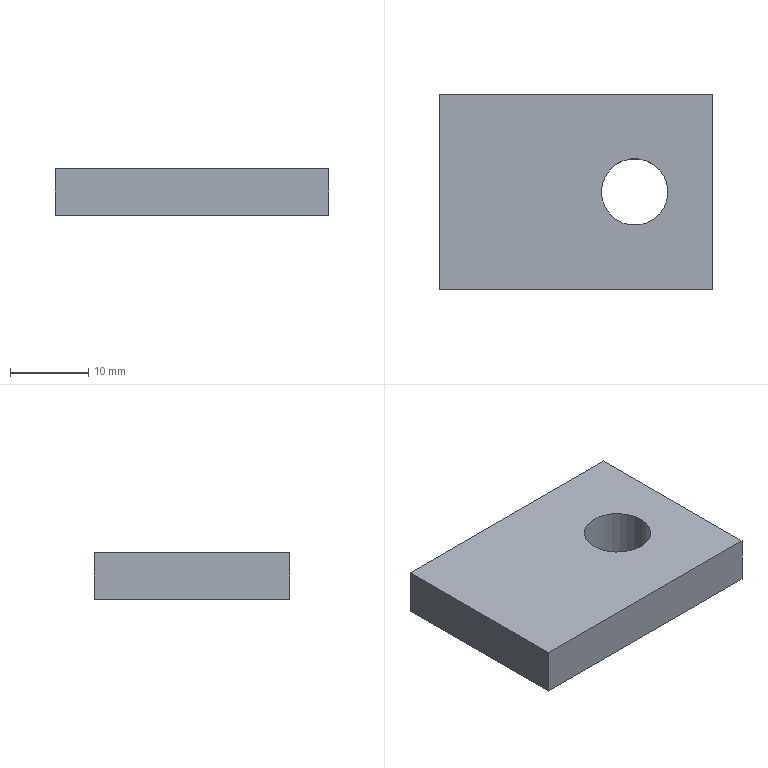Part | SolidWorks | features FlatPattern 1, SMBaseFlange 1, SheetMetal 1 | 1 solid | 8 faces | box 35 x 25 x 6 mm | volume 4910 mm3 | plane 6 | cylinder 2 | commonest cylinder face diameters 8.5 x2
STEP:
#1=CARTESIAN_POINT('',(17908.836,-96147.322,-6.));
#2=VERTEX_POINT('',#1);
#3=CARTESIAN_POINT('',(17917.336,-96147.322,-6.));
#4=VERTEX_POINT('',#3);
#5=CARTESIAN_POINT('',(17913.086,-96147.322,-6.));
#6=DIRECTION('',(0.,0.,1.));
#7=DIRECTION('',(1.,0.,0.));
#8=AXIS2_PLACEMENT_3D('',#5,#6,#7);
#9=CIRCLE('',#8,4.25);
#10=EDGE_CURVE('',#2,#4,#9,.T.);
#11=ORIENTED_EDGE('',*,*,#10,.F.);
#12=CARTESIAN_POINT('',(17908.836,-96147.322,0.));
#13=VERTEX_POINT('',#12);
#14=CARTESIAN_POINT('',(17908.836,-96147.322,-6.));
#15=DIRECTION('',(0.,0.,1.));
#16=VECTOR('',#15,1000.);
#17=LINE('',#14,#16);
#18=EDGE_CURVE('',#2,#13,#17,.T.);
#19=ORIENTED_EDGE('',*,*,#18,.T.);
#20=CARTESIAN_POINT('',(17917.336,-96147.322,0.));
#21=VERTEX_POINT('',#20);
#22=CARTESIAN_POINT('',(17913.086,-96147.322,0.));
#23=DIRECTION('',(0.,0.,1.));
#24=DIRECTION('',(1.,0.,0.));
#25=AXIS2_PLACEMENT_3D('',#22,#23,#24);
#26=CIRCLE('',#25,4.25);
#27=EDGE_CURVE('',#13,#21,#26,.T.);
#28=ORIENTED_EDGE('',*,*,#27,.T.);
#29=CARTESIAN_POINT('',(17917.336,-96147.322,-6.));
#30=DIRECTION('',(0.,0.,1.));
#31=VECTOR('',#30,1000.);
#32=LINE('',#29,#31);
#33=EDGE_CURVE('',#4,#21,#32,.T.);
#34=ORIENTED_EDGE('',*,*,#33,.F.);
#35=EDGE_LOOP('',(#11,#19,#28,#34));
#36=FACE_OUTER_BOUND('',#35,.T.);
#37=CARTESIAN_POINT('',(17913.086,-96147.322,-6.));
#38=DIRECTION('',(0.,0.,1.));
#39=DIRECTION('',(1.,0.,0.));
#40=AXIS2_PLACEMENT_3D('',#37,#38,#39);
#41=CYLINDRICAL_SURFACE('',#40,4.25);
#42=ADVANCED_FACE('',(#36),#41,.F.);
#43=CARTESIAN_POINT('',(17923.086,-96159.822,0.));
#44=VERTEX_POINT('',#43);
#45=CARTESIAN_POINT('',(17923.086,-96134.822,0.));
#46=VERTEX_POINT('',#45);
#47=CARTESIAN_POINT('',(17923.086,-96159.822,0.));
#48=DIRECTION('',(0.,1.,0.));
#49=VECTOR('',#48,1000.);
#50=LINE('',#47,#49);
#51=EDGE_CURVE('',#44,#46,#50,.T.);
#52=ORIENTED_EDGE('',*,*,#51,.F.);
#53=CARTESIAN_POINT('',(17923.086,-96159.822,-6.));
#54=VERTEX_POINT('',#53);
#55=CARTESIAN_POINT('',(17923.086,-96159.822,-6.));
#56=DIRECTION('',(0.,0.,1.));
#57=VECTOR('',#56,1000.);
#58=LINE('',#55,#57);
#59=EDGE_CURVE('',#54,#44,#58,.T.);
#60=ORIENTED_EDGE('',*,*,#59,.F.);
#61=CARTESIAN_POINT('',(17923.086,-96134.822,-6.));
#62=VERTEX_POINT('',#61);
#63=CARTESIAN_POINT('',(17923.086,-96159.822,-6.));
#64=DIRECTION('',(0.,1.,0.));
#65=VECTOR('',#64,1000.);
#66=LINE('',#63,#65);
#67=EDGE_CURVE('',#54,#62,#66,.T.);
#68=ORIENTED_EDGE('',*,*,#67,.T.);
#69=CARTESIAN_POINT('',(17923.086,-96134.822,-6.));
#70=DIRECTION('',(0.,0.,1.));
#71=VECTOR('',#70,1000.);
#72=LINE('',#69,#71);
#73=EDGE_CURVE('',#62,#46,#72,.T.);
#74=ORIENTED_EDGE('',*,*,#73,.T.);
#75=EDGE_LOOP('',(#52,#60,#68,#74));
#76=FACE_OUTER_BOUND('',#75,.T.);
#77=CARTESIAN_POINT('',(17923.086,-96159.822,-6.));
#78=DIRECTION('',(1.,0.,0.));
#79=DIRECTION('',(0.,0.,-1.));
#80=AXIS2_PLACEMENT_3D('',#77,#78,#79);
#81=PLANE('',#80);
#82=ADVANCED_FACE('',(#76),#81,.T.);
#83=CARTESIAN_POINT('',(17888.086,-96159.822,0.));
#84=VERTEX_POINT('',#83);
#85=CARTESIAN_POINT('',(17923.086,-96159.822,0.));
#86=DIRECTION('',(1.,0.,0.));
#87=VECTOR('',#86,1000.);
#88=LINE('',#85,#87);
#89=EDGE_CURVE('',#84,#44,#88,.T.);
#90=ORIENTED_EDGE('',*,*,#89,.F.);
#91=CARTESIAN_POINT('',(17888.086,-96159.822,-6.));
#92=VERTEX_POINT('',#91);
#93=CARTESIAN_POINT('',(17888.086,-96159.822,-6.));
#94=DIRECTION('',(0.,0.,1.));
#95=VECTOR('',#94,1000.);
#96=LINE('',#93,#95);
#97=EDGE_CURVE('',#92,#84,#96,.T.);
#98=ORIENTED_EDGE('',*,*,#97,.F.);
#99=CARTESIAN_POINT('',(17910.456,-96159.822,-6.));
#100=DIRECTION('',(1.,0.,0.));
#101=VECTOR('',#100,1000.);
#102=LINE('',#99,#101);
#103=EDGE_CURVE('',#92,#54,#102,.T.);
#104=ORIENTED_EDGE('',*,*,#103,.T.);
#105=ORIENTED_EDGE('',*,*,#59,.T.);
#106=EDGE_LOOP('',(#90,#98,#104,#105));
#107=FACE_OUTER_BOUND('',#106,.T.);
#108=CARTESIAN_POINT('',(17923.086,-96159.822,-6.));
#109=DIRECTION('',(0.,-1.,0.));
#110=DIRECTION('',(0.,0.,-1.));
#111=AXIS2_PLACEMENT_3D('',#108,#109,#110);
#112=PLANE('',#111);
#113=ADVANCED_FACE('',(#107),#112,.T.);
#114=CARTESIAN_POINT('',(17888.086,-96134.822,0.));
#115=VERTEX_POINT('',#114);
#116=CARTESIAN_POINT('',(17888.086,-96159.822,0.));
#117=DIRECTION('',(0.,-1.,0.));
#118=VECTOR('',#117,1000.);
#119=LINE('',#116,#118);
#120=EDGE_CURVE('',#115,#84,#119,.T.);
#121=ORIENTED_EDGE('',*,*,#120,.F.);
#122=CARTESIAN_POINT('',(17888.086,-96134.822,-6.));
#123=VERTEX_POINT('',#122);
#124=CARTESIAN_POINT('',(17888.086,-96134.822,-6.));
#125=DIRECTION('',(0.,0.,1.));
#126=VECTOR('',#125,1000.);
#127=LINE('',#124,#126);
#128=EDGE_CURVE('',#123,#115,#127,.T.);
#129=ORIENTED_EDGE('',*,*,#128,.F.);
#130=CARTESIAN_POINT('',(17888.086,-96159.822,-6.));
#131=DIRECTION('',(0.,-1.,0.));
#132=VECTOR('',#131,1000.);
#133=LINE('',#130,#132);
#134=EDGE_CURVE('',#123,#92,#133,.T.);
#135=ORIENTED_EDGE('',*,*,#134,.T.);
#136=ORIENTED_EDGE('',*,*,#97,.T.);
#137=EDGE_LOOP('',(#121,#129,#135,#136));
#138=FACE_OUTER_BOUND('',#137,.T.);
#139=CARTESIAN_POINT('',(17888.086,-96159.822,-6.));
#140=DIRECTION('',(-1.,0.,0.));
#141=DIRECTION('',(0.,0.,1.));
#142=AXIS2_PLACEMENT_3D('',#139,#140,#141);
#143=PLANE('',#142);
#144=ADVANCED_FACE('',(#138),#143,.T.);
#145=CARTESIAN_POINT('',(17910.269,-96134.822,0.));
#146=DIRECTION('',(-1.,0.,0.));
#147=VECTOR('',#146,1000.);
#148=LINE('',#145,#147);
#149=EDGE_CURVE('',#46,#115,#148,.T.);
#150=ORIENTED_EDGE('',*,*,#149,.F.);
#151=ORIENTED_EDGE('',*,*,#73,.F.);
#152=CARTESIAN_POINT('',(17923.086,-96134.822,-6.));
#153=DIRECTION('',(-1.,0.,0.));
#154=VECTOR('',#153,1000.);
#155=LINE('',#152,#154);
#156=EDGE_CURVE('',#62,#123,#155,.T.);
#157=ORIENTED_EDGE('',*,*,#156,.T.);
#158=ORIENTED_EDGE('',*,*,#128,.T.);
#159=EDGE_LOOP('',(#150,#151,#157,#158));
#160=FACE_OUTER_BOUND('',#159,.T.);
#161=CARTESIAN_POINT('',(17910.269,-96134.822,-6.));
#162=DIRECTION('',(0.,1.,0.));
#163=DIRECTION('',(0.,0.,1.));
#164=AXIS2_PLACEMENT_3D('',#161,#162,#163);
#165=PLANE('',#164);
#166=ADVANCED_FACE('',(#160),#165,.T.);
#167=CARTESIAN_POINT('',(17913.086,-96147.322,-6.));
#168=DIRECTION('',(0.,0.,1.));
#169=DIRECTION('',(1.,0.,0.));
#170=AXIS2_PLACEMENT_3D('',#167,#168,#169);
#171=CIRCLE('',#170,4.25);
#172=EDGE_CURVE('',#4,#2,#171,.T.);
#173=ORIENTED_EDGE('',*,*,#172,.T.);
#174=ORIENTED_EDGE('',*,*,#10,.T.);
#175=EDGE_LOOP('',(#173,#174));
#176=FACE_BOUND('',#175,.T.);
#177=ORIENTED_EDGE('',*,*,#67,.F.);
#178=ORIENTED_EDGE('',*,*,#103,.F.);
#179=ORIENTED_EDGE('',*,*,#134,.F.);
#180=ORIENTED_EDGE('',*,*,#156,.F.);
#181=EDGE_LOOP('',(#177,#178,#179,#180));
#182=FACE_OUTER_BOUND('',#181,.T.);
#183=CARTESIAN_POINT('',(0.,0.,-6.));
#184=DIRECTION('',(0.,0.,1.));
#185=DIRECTION('',(1.,0.,0.));
#186=AXIS2_PLACEMENT_3D('',#183,#184,#185);
#187=PLANE('',#186);
#188=ADVANCED_FACE('',(#176,#182),#187,.F.);
#189=CARTESIAN_POINT('',(17913.086,-96147.322,0.));
#190=DIRECTION('',(0.,0.,1.));
#191=DIRECTION('',(1.,0.,0.));
#192=AXIS2_PLACEMENT_3D('',#189,#190,#191);
#193=CIRCLE('',#192,4.25);
#194=EDGE_CURVE('',#21,#13,#193,.T.);
#195=ORIENTED_EDGE('',*,*,#194,.F.);
#196=ORIENTED_EDGE('',*,*,#27,.F.);
#197=EDGE_LOOP('',(#195,#196));
#198=FACE_BOUND('',#197,.T.);
#199=ORIENTED_EDGE('',*,*,#51,.T.);
#200=ORIENTED_EDGE('',*,*,#149,.T.);
#201=ORIENTED_EDGE('',*,*,#120,.T.);
#202=ORIENTED_EDGE('',*,*,#89,.T.);
#203=EDGE_LOOP('',(#199,#200,#201,#202));
#204=FACE_OUTER_BOUND('',#203,.T.);
#205=CARTESIAN_POINT('',(0.,0.,0.));
#206=DIRECTION('',(0.,0.,1.));
#207=DIRECTION('',(1.,0.,0.));
#208=AXIS2_PLACEMENT_3D('',#205,#206,#207);
#209=PLANE('',#208);
#210=ADVANCED_FACE('',(#198,#204),#209,.T.);
#211=ORIENTED_EDGE('',*,*,#18,.F.);
#212=ORIENTED_EDGE('',*,*,#172,.F.);
#213=ORIENTED_EDGE('',*,*,#33,.T.);
#214=ORIENTED_EDGE('',*,*,#194,.T.);
#215=EDGE_LOOP('',(#211,#212,#213,#214));
#216=FACE_OUTER_BOUND('',#215,.T.);
#217=CARTESIAN_POINT('',(17913.086,-96147.322,-6.));
#218=DIRECTION('',(0.,0.,1.));
#219=DIRECTION('',(1.,0.,0.));
#220=AXIS2_PLACEMENT_3D('',#217,#218,#219);
#221=CYLINDRICAL_SURFACE('',#220,4.25);
#222=ADVANCED_FACE('',(#216),#221,.F.);
#223=CLOSED_SHELL('',(#42,#82,#113,#144,#166,#188,#210,#222));
#224=MANIFOLD_SOLID_BREP('',#223);
#225=CARTESIAN_POINT('',(0.,0.,0.));
#226=DIRECTION('',(0.,0.,1.));
#227=DIRECTION('',(1.,0.,0.));
#228=AXIS2_PLACEMENT_3D('',#225,#226,#227);
#229=(LENGTH_UNIT()NAMED_UNIT(*)SI_UNIT(.MILLI.,.METRE.));
#230=UNCERTAINTY_MEASURE_WITH_UNIT(LENGTH_MEASURE(0.00001),#229,'','');
#231=(NAMED_UNIT(*)PLANE_ANGLE_UNIT()SI_UNIT($,.RADIAN.));
#232=(NAMED_UNIT(*)SI_UNIT($,.STERADIAN.)SOLID_ANGLE_UNIT());
#233=(GEOMETRIC_REPRESENTATION_CONTEXT(3)GLOBAL_UNCERTAINTY_ASSIGNED_CONTEXT((#230))GLOBAL_UNIT_ASSIGNED_CONTEXT((#229,#231,#232))REPRESENTATION_CONTEXT('',''));
#234=ADVANCED_BREP_SHAPE_REPRESENTATION('',(#224,#228),#233);